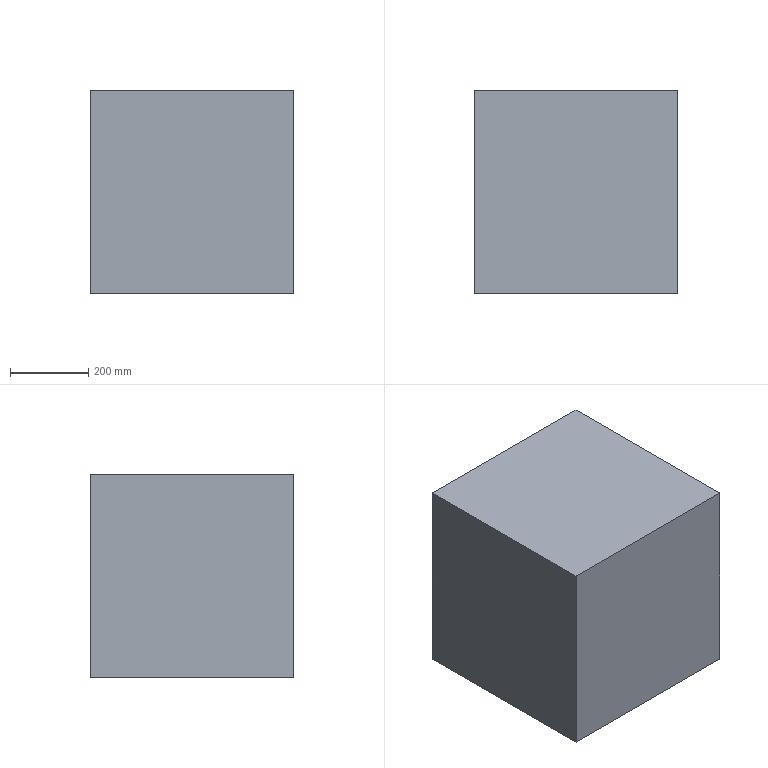Part | SolidWorks | features ICE 2, BaseBody 1 | 1 solid | 44 faces | box 520 x 520 x 520 mm | volume 15406938 mm3 | cylinder 32 | plane 12 | commonest cylinder face diameters 40 x32
STEP:
#1=CARTESIAN_POINT('',(400.507,102.938,240.));
#2=VERTEX_POINT('',#1);
#3=CARTESIAN_POINT('',(400.507,102.938,200.));
#4=VERTEX_POINT('',#3);
#5=CARTESIAN_POINT('',(400.507,102.938,220.));
#6=DIRECTION('',(1.,0.,0.));
#7=DIRECTION('',(0.,0.,-1.));
#8=AXIS2_PLACEMENT_3D('',#5,#6,#7);
#9=CIRCLE('',#8,20.);
#10=EDGE_CURVE('',#2,#4,#9,.T.);
#11=ORIENTED_EDGE('',*,*,#10,.F.);
#12=CARTESIAN_POINT('',(410.507,102.938,240.));
#13=VERTEX_POINT('',#12);
#14=CARTESIAN_POINT('',(400.507,102.938,240.));
#15=DIRECTION('',(1.,0.,0.));
#16=VECTOR('',#15,1000.);
#17=LINE('',#14,#16);
#18=EDGE_CURVE('',#2,#13,#17,.T.);
#19=ORIENTED_EDGE('',*,*,#18,.T.);
#20=CARTESIAN_POINT('',(410.507,102.938,200.));
#21=VERTEX_POINT('',#20);
#22=CARTESIAN_POINT('',(410.507,102.938,220.));
#23=DIRECTION('',(1.,0.,0.));
#24=DIRECTION('',(0.,0.,-1.));
#25=AXIS2_PLACEMENT_3D('',#22,#23,#24);
#26=CIRCLE('',#25,20.);
#27=EDGE_CURVE('',#13,#21,#26,.T.);
#28=ORIENTED_EDGE('',*,*,#27,.T.);
#29=CARTESIAN_POINT('',(400.507,102.938,200.));
#30=DIRECTION('',(1.,0.,0.));
#31=VECTOR('',#30,1000.);
#32=LINE('',#29,#31);
#33=EDGE_CURVE('',#4,#21,#32,.T.);
#34=ORIENTED_EDGE('',*,*,#33,.F.);
#35=EDGE_LOOP('',(#11,#19,#28,#34));
#36=FACE_OUTER_BOUND('',#35,.T.);
#37=CARTESIAN_POINT('',(400.507,102.938,220.));
#38=DIRECTION('',(1.,0.,0.));
#39=DIRECTION('',(0.,0.,-1.));
#40=AXIS2_PLACEMENT_3D('',#37,#38,#39);
#41=CYLINDRICAL_SURFACE('',#40,20.);
#42=ADVANCED_FACE('',(#36),#41,.F.);
#43=CARTESIAN_POINT('',(400.507,102.938,340.));
#44=VERTEX_POINT('',#43);
#45=CARTESIAN_POINT('',(400.507,102.938,300.));
#46=VERTEX_POINT('',#45);
#47=CARTESIAN_POINT('',(400.507,102.938,320.));
#48=DIRECTION('',(1.,0.,0.));
#49=DIRECTION('',(0.,0.,-1.));
#50=AXIS2_PLACEMENT_3D('',#47,#48,#49);
#51=CIRCLE('',#50,20.);
#52=EDGE_CURVE('',#44,#46,#51,.T.);
#53=ORIENTED_EDGE('',*,*,#52,.F.);
#54=CARTESIAN_POINT('',(410.507,102.938,340.));
#55=VERTEX_POINT('',#54);
#56=CARTESIAN_POINT('',(400.507,102.938,340.));
#57=DIRECTION('',(1.,0.,0.));
#58=VECTOR('',#57,1000.);
#59=LINE('',#56,#58);
#60=EDGE_CURVE('',#44,#55,#59,.T.);
#61=ORIENTED_EDGE('',*,*,#60,.T.);
#62=CARTESIAN_POINT('',(410.507,102.938,300.));
#63=VERTEX_POINT('',#62);
#64=CARTESIAN_POINT('',(410.507,102.938,320.));
#65=DIRECTION('',(1.,0.,0.));
#66=DIRECTION('',(0.,0.,-1.));
#67=AXIS2_PLACEMENT_3D('',#64,#65,#66);
#68=CIRCLE('',#67,20.);
#69=EDGE_CURVE('',#55,#63,#68,.T.);
#70=ORIENTED_EDGE('',*,*,#69,.T.);
#71=CARTESIAN_POINT('',(400.507,102.938,300.));
#72=DIRECTION('',(1.,0.,0.));
#73=VECTOR('',#72,1000.);
#74=LINE('',#71,#73);
#75=EDGE_CURVE('',#46,#63,#74,.T.);
#76=ORIENTED_EDGE('',*,*,#75,.F.);
#77=EDGE_LOOP('',(#53,#61,#70,#76));
#78=FACE_OUTER_BOUND('',#77,.T.);
#79=CARTESIAN_POINT('',(400.507,102.938,320.));
#80=DIRECTION('',(1.,0.,0.));
#81=DIRECTION('',(0.,0.,-1.));
#82=AXIS2_PLACEMENT_3D('',#79,#80,#81);
#83=CYLINDRICAL_SURFACE('',#82,20.);
#84=ADVANCED_FACE('',(#78),#83,.F.);
#85=CARTESIAN_POINT('',(400.507,-97.062,440.));
#86=VERTEX_POINT('',#85);
#87=CARTESIAN_POINT('',(400.507,-97.062,400.));
#88=VERTEX_POINT('',#87);
#89=CARTESIAN_POINT('',(400.507,-97.062,420.));
#90=DIRECTION('',(1.,0.,0.));
#91=DIRECTION('',(0.,0.,-1.));
#92=AXIS2_PLACEMENT_3D('',#89,#90,#91);
#93=CIRCLE('',#92,20.);
#94=EDGE_CURVE('',#86,#88,#93,.T.);
#95=ORIENTED_EDGE('',*,*,#94,.F.);
#96=CARTESIAN_POINT('',(410.507,-97.062,440.));
#97=VERTEX_POINT('',#96);
#98=CARTESIAN_POINT('',(400.507,-97.062,440.));
#99=DIRECTION('',(1.,0.,0.));
#100=VECTOR('',#99,1000.);
#101=LINE('',#98,#100);
#102=EDGE_CURVE('',#86,#97,#101,.T.);
#103=ORIENTED_EDGE('',*,*,#102,.T.);
#104=CARTESIAN_POINT('',(410.507,-97.062,400.));
#105=VERTEX_POINT('',#104);
#106=CARTESIAN_POINT('',(410.507,-97.062,420.));
#107=DIRECTION('',(1.,0.,0.));
#108=DIRECTION('',(0.,0.,-1.));
#109=AXIS2_PLACEMENT_3D('',#106,#107,#108);
#110=CIRCLE('',#109,20.);
#111=EDGE_CURVE('',#97,#105,#110,.T.);
#112=ORIENTED_EDGE('',*,*,#111,.T.);
#113=CARTESIAN_POINT('',(400.507,-97.062,400.));
#114=DIRECTION('',(1.,0.,0.));
#115=VECTOR('',#114,1000.);
#116=LINE('',#113,#115);
#117=EDGE_CURVE('',#88,#105,#116,.T.);
#118=ORIENTED_EDGE('',*,*,#117,.F.);
#119=EDGE_LOOP('',(#95,#103,#112,#118));
#120=FACE_OUTER_BOUND('',#119,.T.);
#121=CARTESIAN_POINT('',(400.507,-97.062,420.));
#122=DIRECTION('',(1.,0.,0.));
#123=DIRECTION('',(0.,0.,-1.));
#124=AXIS2_PLACEMENT_3D('',#121,#122,#123);
#125=CYLINDRICAL_SURFACE('',#124,20.);
#126=ADVANCED_FACE('',(#120),#125,.F.);
#127=CARTESIAN_POINT('',(400.507,2.938,440.));
#128=VERTEX_POINT('',#127);
#129=CARTESIAN_POINT('',(400.507,2.938,400.));
#130=VERTEX_POINT('',#129);
#131=CARTESIAN_POINT('',(400.507,2.938,420.));
#132=DIRECTION('',(1.,0.,0.));
#133=DIRECTION('',(0.,0.,-1.));
#134=AXIS2_PLACEMENT_3D('',#131,#132,#133);
#135=CIRCLE('',#134,20.);
#136=EDGE_CURVE('',#128,#130,#135,.T.);
#137=ORIENTED_EDGE('',*,*,#136,.F.);
#138=CARTESIAN_POINT('',(410.507,2.938,440.));
#139=VERTEX_POINT('',#138);
#140=CARTESIAN_POINT('',(400.507,2.938,440.));
#141=DIRECTION('',(1.,0.,0.));
#142=VECTOR('',#141,1000.);
#143=LINE('',#140,#142);
#144=EDGE_CURVE('',#128,#139,#143,.T.);
#145=ORIENTED_EDGE('',*,*,#144,.T.);
#146=CARTESIAN_POINT('',(410.507,2.938,400.));
#147=VERTEX_POINT('',#146);
#148=CARTESIAN_POINT('',(410.507,2.938,420.));
#149=DIRECTION('',(1.,0.,0.));
#150=DIRECTION('',(0.,0.,-1.));
#151=AXIS2_PLACEMENT_3D('',#148,#149,#150);
#152=CIRCLE('',#151,20.);
#153=EDGE_CURVE('',#139,#147,#152,.T.);
#154=ORIENTED_EDGE('',*,*,#153,.T.);
#155=CARTESIAN_POINT('',(400.507,2.938,400.));
#156=DIRECTION('',(1.,0.,0.));
#157=VECTOR('',#156,1000.);
#158=LINE('',#155,#157);
#159=EDGE_CURVE('',#130,#147,#158,.T.);
#160=ORIENTED_EDGE('',*,*,#159,.F.);
#161=EDGE_LOOP('',(#137,#145,#154,#160));
#162=FACE_OUTER_BOUND('',#161,.T.);
#163=CARTESIAN_POINT('',(400.507,2.938,420.));
#164=DIRECTION('',(1.,0.,0.));
#165=DIRECTION('',(0.,0.,-1.));
#166=AXIS2_PLACEMENT_3D('',#163,#164,#165);
#167=CYLINDRICAL_SURFACE('',#166,20.);
#168=ADVANCED_FACE('',(#162),#167,.F.);
#169=CARTESIAN_POINT('',(400.507,202.938,340.));
#170=VERTEX_POINT('',#169);
#171=CARTESIAN_POINT('',(400.507,202.938,300.));
#172=VERTEX_POINT('',#171);
#173=CARTESIAN_POINT('',(400.507,202.938,320.));
#174=DIRECTION('',(1.,0.,0.));
#175=DIRECTION('',(0.,0.,-1.));
#176=AXIS2_PLACEMENT_3D('',#173,#174,#175);
#177=CIRCLE('',#176,20.);
#178=EDGE_CURVE('',#170,#172,#177,.T.);
#179=ORIENTED_EDGE('',*,*,#178,.F.);
#180=CARTESIAN_POINT('',(410.507,202.938,340.));
#181=VERTEX_POINT('',#180);
#182=CARTESIAN_POINT('',(400.507,202.938,340.));
#183=DIRECTION('',(1.,0.,0.));
#184=VECTOR('',#183,1000.);
#185=LINE('',#182,#184);
#186=EDGE_CURVE('',#170,#181,#185,.T.);
#187=ORIENTED_EDGE('',*,*,#186,.T.);
#188=CARTESIAN_POINT('',(410.507,202.938,300.));
#189=VERTEX_POINT('',#188);
#190=CARTESIAN_POINT('',(410.507,202.938,320.));
#191=DIRECTION('',(1.,0.,0.));
#192=DIRECTION('',(0.,0.,-1.));
#193=AXIS2_PLACEMENT_3D('',#190,#191,#192);
#194=CIRCLE('',#193,20.);
#195=EDGE_CURVE('',#181,#189,#194,.T.);
#196=ORIENTED_EDGE('',*,*,#195,.T.);
#197=CARTESIAN_POINT('',(400.507,202.938,300.));
#198=DIRECTION('',(1.,0.,0.));
#199=VECTOR('',#198,1000.);
#200=LINE('',#197,#199);
#201=EDGE_CURVE('',#172,#189,#200,.T.);
#202=ORIENTED_EDGE('',*,*,#201,.F.);
#203=EDGE_LOOP('',(#179,#187,#196,#202));
#204=FACE_OUTER_BOUND('',#203,.T.);
#205=CARTESIAN_POINT('',(400.507,202.938,320.));
#206=DIRECTION('',(1.,0.,0.));
#207=DIRECTION('',(0.,0.,-1.));
#208=AXIS2_PLACEMENT_3D('',#205,#206,#207);
#209=CYLINDRICAL_SURFACE('',#208,20.);
#210=ADVANCED_FACE('',(#204),#209,.F.);
#211=CARTESIAN_POINT('',(400.507,202.938,240.));
#212=VERTEX_POINT('',#211);
#213=CARTESIAN_POINT('',(400.507,202.938,200.));
#214=VERTEX_POINT('',#213);
#215=CARTESIAN_POINT('',(400.507,202.938,220.));
#216=DIRECTION('',(1.,0.,0.));
#217=DIRECTION('',(0.,0.,-1.));
#218=AXIS2_PLACEMENT_3D('',#215,#216,#217);
#219=CIRCLE('',#218,20.);
#220=EDGE_CURVE('',#212,#214,#219,.T.);
#221=ORIENTED_EDGE('',*,*,#220,.F.);
#222=CARTESIAN_POINT('',(410.507,202.938,240.));
#223=VERTEX_POINT('',#222);
#224=CARTESIAN_POINT('',(400.507,202.938,240.));
#225=DIRECTION('',(1.,0.,0.));
#226=VECTOR('',#225,1000.);
#227=LINE('',#224,#226);
#228=EDGE_CURVE('',#212,#223,#227,.T.);
#229=ORIENTED_EDGE('',*,*,#228,.T.);
#230=CARTESIAN_POINT('',(410.507,202.938,200.));
#231=VERTEX_POINT('',#230);
#232=CARTESIAN_POINT('',(410.507,202.938,220.));
#233=DIRECTION('',(1.,0.,0.));
#234=DIRECTION('',(0.,0.,-1.));
#235=AXIS2_PLACEMENT_3D('',#232,#233,#234);
#236=CIRCLE('',#235,20.);
#237=EDGE_CURVE('',#223,#231,#236,.T.);
#238=ORIENTED_EDGE('',*,*,#237,.T.);
#239=CARTESIAN_POINT('',(400.507,202.938,200.));
#240=DIRECTION('',(1.,0.,0.));
#241=VECTOR('',#240,1000.);
#242=LINE('',#239,#241);
#243=EDGE_CURVE('',#214,#231,#242,.T.);
#244=ORIENTED_EDGE('',*,*,#243,.F.);
#245=EDGE_LOOP('',(#221,#229,#238,#244));
#246=FACE_OUTER_BOUND('',#245,.T.);
#247=CARTESIAN_POINT('',(400.507,202.938,220.));
#248=DIRECTION('',(1.,0.,0.));
#249=DIRECTION('',(0.,0.,-1.));
#250=AXIS2_PLACEMENT_3D('',#247,#248,#249);
#251=CYLINDRICAL_SURFACE('',#250,20.);
#252=ADVANCED_FACE('',(#246),#251,.F.);
#253=CARTESIAN_POINT('',(400.507,202.938,140.));
#254=VERTEX_POINT('',#253);
#255=CARTESIAN_POINT('',(400.507,202.938,100.));
#256=VERTEX_POINT('',#255);
#257=CARTESIAN_POINT('',(400.507,202.938,120.));
#258=DIRECTION('',(1.,0.,0.));
#259=DIRECTION('',(0.,0.,-1.));
#260=AXIS2_PLACEMENT_3D('',#257,#258,#259);
#261=CIRCLE('',#260,20.);
#262=EDGE_CURVE('',#254,#256,#261,.T.);
#263=ORIENTED_EDGE('',*,*,#262,.F.);
#264=CARTESIAN_POINT('',(410.507,202.938,140.));
#265=VERTEX_POINT('',#264);
#266=CARTESIAN_POINT('',(400.507,202.938,140.));
#267=DIRECTION('',(1.,0.,0.));
#268=VECTOR('',#267,1000.);
#269=LINE('',#266,#268);
#270=EDGE_CURVE('',#254,#265,#269,.T.);
#271=ORIENTED_EDGE('',*,*,#270,.T.);
#272=CARTESIAN_POINT('',(410.507,202.938,100.));
#273=VERTEX_POINT('',#272);
#274=CARTESIAN_POINT('',(410.507,202.938,120.));
#275=DIRECTION('',(1.,0.,0.));
#276=DIRECTION('',(0.,0.,-1.));
#277=AXIS2_PLACEMENT_3D('',#274,#275,#276);
#278=CIRCLE('',#277,20.);
#279=EDGE_CURVE('',#265,#273,#278,.T.);
#280=ORIENTED_EDGE('',*,*,#279,.T.);
#281=CARTESIAN_POINT('',(400.507,202.938,100.));
#282=DIRECTION('',(1.,0.,0.));
#283=VECTOR('',#282,1000.);
#284=LINE('',#281,#283);
#285=EDGE_CURVE('',#256,#273,#284,.T.);
#286=ORIENTED_EDGE('',*,*,#285,.F.);
#287=EDGE_LOOP('',(#263,#271,#280,#286));
#288=FACE_OUTER_BOUND('',#287,.T.);
#289=CARTESIAN_POINT('',(400.507,202.938,120.));
#290=DIRECTION('',(1.,0.,0.));
#291=DIRECTION('',(0.,0.,-1.));
#292=AXIS2_PLACEMENT_3D('',#289,#290,#291);
#293=CYLINDRICAL_SURFACE('',#292,20.);
#294=ADVANCED_FACE('',(#288),#293,.F.);
#295=CARTESIAN_POINT('',(400.507,102.938,440.));
#296=VERTEX_POINT('',#295);
#297=CARTESIAN_POINT('',(400.507,102.938,400.));
#298=VERTEX_POINT('',#297);
#299=CARTESIAN_POINT('',(400.507,102.938,420.));
#300=DIRECTION('',(1.,0.,0.));
#301=DIRECTION('',(0.,0.,-1.));
#302=AXIS2_PLACEMENT_3D('',#299,#300,#301);
#303=CIRCLE('',#302,20.);
#304=EDGE_CURVE('',#296,#298,#303,.T.);
#305=ORIENTED_EDGE('',*,*,#304,.F.);
#306=CARTESIAN_POINT('',(410.507,102.938,440.));
#307=VERTEX_POINT('',#306);
#308=CARTESIAN_POINT('',(400.507,102.938,440.));
#309=DIRECTION('',(1.,0.,0.));
#310=VECTOR('',#309,1000.);
#311=LINE('',#308,#310);
#312=EDGE_CURVE('',#296,#307,#311,.T.);
#313=ORIENTED_EDGE('',*,*,#312,.T.);
#314=CARTESIAN_POINT('',(410.507,102.938,400.));
#315=VERTEX_POINT('',#314);
#316=CARTESIAN_POINT('',(410.507,102.938,420.));
#317=DIRECTION('',(1.,0.,0.));
#318=DIRECTION('',(0.,0.,-1.));
#319=AXIS2_PLACEMENT_3D('',#316,#317,#318);
#320=CIRCLE('',#319,20.);
#321=EDGE_CURVE('',#307,#315,#320,.T.);
#322=ORIENTED_EDGE('',*,*,#321,.T.);
#323=CARTESIAN_POINT('',(400.507,102.938,400.));
#324=DIRECTION('',(1.,0.,0.));
#325=VECTOR('',#324,1000.);
#326=LINE('',#323,#325);
#327=EDGE_CURVE('',#298,#315,#326,.T.);
#328=ORIENTED_EDGE('',*,*,#327,.F.);
#329=EDGE_LOOP('',(#305,#313,#322,#328));
#330=FACE_OUTER_BOUND('',#329,.T.);
#331=CARTESIAN_POINT('',(400.507,102.938,420.));
#332=DIRECTION('',(1.,0.,0.));
#333=DIRECTION('',(0.,0.,-1.));
#334=AXIS2_PLACEMENT_3D('',#331,#332,#333);
#335=CYLINDRICAL_SURFACE('',#334,20.);
#336=ADVANCED_FACE('',(#330),#335,.F.);
#337=CARTESIAN_POINT('',(400.507,2.938,140.));
#338=VERTEX_POINT('',#337);
#339=CARTESIAN_POINT('',(400.507,2.938,100.));
#340=VERTEX_POINT('',#339);
#341=CARTESIAN_POINT('',(400.507,2.938,120.));
#342=DIRECTION('',(1.,0.,0.));
#343=DIRECTION('',(0.,0.,-1.));
#344=AXIS2_PLACEMENT_3D('',#341,#342,#343);
#345=CIRCLE('',#344,20.);
#346=EDGE_CURVE('',#338,#340,#345,.T.);
#347=ORIENTED_EDGE('',*,*,#346,.F.);
#348=CARTESIAN_POINT('',(410.507,2.938,140.));
#349=VERTEX_POINT('',#348);
#350=CARTESIAN_POINT('',(400.507,2.938,140.));
#351=DIRECTION('',(1.,0.,0.));
#352=VECTOR('',#351,1000.);
#353=LINE('',#350,#352);
#354=EDGE_CURVE('',#338,#349,#353,.T.);
#355=ORIENTED_EDGE('',*,*,#354,.T.);
#356=CARTESIAN_POINT('',(410.507,2.938,100.));
#357=VERTEX_POINT('',#356);
#358=CARTESIAN_POINT('',(410.507,2.938,120.));
#359=DIRECTION('',(1.,0.,0.));
#360=DIRECTION('',(0.,0.,-1.));
#361=AXIS2_PLACEMENT_3D('',#358,#359,#360);
#362=CIRCLE('',#361,20.);
#363=EDGE_CURVE('',#349,#357,#362,.T.);
#364=ORIENTED_EDGE('',*,*,#363,.T.);
#365=CARTESIAN_POINT('',(400.507,2.938,100.));
#366=DIRECTION('',(1.,0.,0.));
#367=VECTOR('',#366,1000.);
#368=LINE('',#365,#367);
#369=EDGE_CURVE('',#340,#357,#368,.T.);
#370=ORIENTED_EDGE('',*,*,#369,.F.);
#371=EDGE_LOOP('',(#347,#355,#364,#370));
#372=FACE_OUTER_BOUND('',#371,.T.);
#373=CARTESIAN_POINT('',(400.507,2.938,120.));
#374=DIRECTION('',(1.,0.,0.));
#375=DIRECTION('',(0.,0.,-1.));
#376=AXIS2_PLACEMENT_3D('',#373,#374,#375);
#377=CYLINDRICAL_SURFACE('',#376,20.);
#378=ADVANCED_FACE('',(#372),#377,.F.);
#379=CARTESIAN_POINT('',(400.507,2.938,240.));
#380=VERTEX_POINT('',#379);
#381=CARTESIAN_POINT('',(400.507,2.938,200.));
#382=VERTEX_POINT('',#381);
#383=CARTESIAN_POINT('',(400.507,2.938,220.));
#384=DIRECTION('',(1.,0.,0.));
#385=DIRECTION('',(0.,0.,-1.));
#386=AXIS2_PLACEMENT_3D('',#383,#384,#385);
#387=CIRCLE('',#386,20.);
#388=EDGE_CURVE('',#380,#382,#387,.T.);
#389=ORIENTED_EDGE('',*,*,#388,.F.);
#390=CARTESIAN_POINT('',(410.507,2.938,240.));
#391=VERTEX_POINT('',#390);
#392=CARTESIAN_POINT('',(400.507,2.938,240.));
#393=DIRECTION('',(1.,0.,0.));
#394=VECTOR('',#393,1000.);
#395=LINE('',#392,#394);
#396=EDGE_CURVE('',#380,#391,#395,.T.);
#397=ORIENTED_EDGE('',*,*,#396,.T.);
#398=CARTESIAN_POINT('',(410.507,2.938,200.));
#399=VERTEX_POINT('',#398);
#400=CARTESIAN_POINT('',(410.507,2.938,220.));
#401=DIRECTION('',(1.,0.,0.));
#402=DIRECTION('',(0.,0.,-1.));
#403=AXIS2_PLACEMENT_3D('',#400,#401,#402);
#404=CIRCLE('',#403,20.);
#405=EDGE_CURVE('',#391,#399,#404,.T.);
#406=ORIENTED_EDGE('',*,*,#405,.T.);
#407=CARTESIAN_POINT('',(400.507,2.938,200.));
#408=DIRECTION('',(1.,0.,0.));
#409=VECTOR('',#408,1000.);
#410=LINE('',#407,#409);
#411=EDGE_CURVE('',#382,#399,#410,.T.);
#412=ORIENTED_EDGE('',*,*,#411,.F.);
#413=EDGE_LOOP('',(#389,#397,#406,#412));
#414=FACE_OUTER_BOUND('',#413,.T.);
#415=CARTESIAN_POINT('',(400.507,2.938,220.));
#416=DIRECTION('',(1.,0.,0.));
#417=DIRECTION('',(0.,0.,-1.));
#418=AXIS2_PLACEMENT_3D('',#415,#416,#417);
#419=CYLINDRICAL_SURFACE('',#418,20.);
#420=ADVANCED_FACE('',(#414),#419,.F.);
#421=CARTESIAN_POINT('',(400.507,2.938,340.));
#422=VERTEX_POINT('',#421);
#423=CARTESIAN_POINT('',(400.507,2.938,300.));
#424=VERTEX_POINT('',#423);
#425=CARTESIAN_POINT('',(400.507,2.938,320.));
#426=DIRECTION('',(1.,0.,0.));
#427=DIRECTION('',(0.,0.,-1.));
#428=AXIS2_PLACEMENT_3D('',#425,#426,#427);
#429=CIRCLE('',#428,20.);
#430=EDGE_CURVE('',#422,#424,#429,.T.);
#431=ORIENTED_EDGE('',*,*,#430,.F.);
#432=CARTESIAN_POINT('',(410.507,2.938,340.));
#433=VERTEX_POINT('',#432);
#434=CARTESIAN_POINT('',(400.507,2.938,340.));
#435=DIRECTION('',(1.,0.,0.));
#436=VECTOR('',#435,1000.);
#437=LINE('',#434,#436);
#438=EDGE_CURVE('',#422,#433,#437,.T.);
#439=ORIENTED_EDGE('',*,*,#438,.T.);
#440=CARTESIAN_POINT('',(410.507,2.938,300.));
#441=VERTEX_POINT('',#440);
#442=CARTESIAN_POINT('',(410.507,2.938,320.));
#443=DIRECTION('',(1.,0.,0.));
#444=DIRECTION('',(0.,0.,-1.));
#445=AXIS2_PLACEMENT_3D('',#442,#443,#444);
#446=CIRCLE('',#445,20.);
#447=EDGE_CURVE('',#433,#441,#446,.T.);
#448=ORIENTED_EDGE('',*,*,#447,.T.);
#449=CARTESIAN_POINT('',(400.507,2.938,300.));
#450=DIRECTION('',(1.,0.,0.));
#451=VECTOR('',#450,1000.);
#452=LINE('',#449,#451);
#453=EDGE_CURVE('',#424,#441,#452,.T.);
#454=ORIENTED_EDGE('',*,*,#453,.F.);
#455=EDGE_LOOP('',(#431,#439,#448,#454));
#456=FACE_OUTER_BOUND('',#455,.T.);
#457=CARTESIAN_POINT('',(400.507,2.938,320.));
#458=DIRECTION('',(1.,0.,0.));
#459=DIRECTION('',(0.,0.,-1.));
#460=AXIS2_PLACEMENT_3D('',#457,#458,#459);
#461=CYLINDRICAL_SURFACE('',#460,20.);
#462=ADVANCED_FACE('',(#456),#461,.F.);
#463=CARTESIAN_POINT('',(400.507,102.938,140.));
#464=VERTEX_POINT('',#463);
#465=CARTESIAN_POINT('',(400.507,102.938,100.));
#466=VERTEX_POINT('',#465);
#467=CARTESIAN_POINT('',(400.507,102.938,120.));
#468=DIRECTION('',(1.,0.,0.));
#469=DIRECTION('',(0.,0.,-1.));
#470=AXIS2_PLACEMENT_3D('',#467,#468,#469);
#471=CIRCLE('',#470,20.);
#472=EDGE_CURVE('',#464,#466,#471,.T.);
#473=ORIENTED_EDGE('',*,*,#472,.F.);
#474=CARTESIAN_POINT('',(410.507,102.938,140.));
#475=VERTEX_POINT('',#474);
#476=CARTESIAN_POINT('',(400.507,102.938,140.));
#477=DIRECTION('',(1.,0.,0.));
#478=VECTOR('',#477,1000.);
#479=LINE('',#476,#478);
#480=EDGE_CURVE('',#464,#475,#479,.T.);
#481=ORIENTED_EDGE('',*,*,#480,.T.);
#482=CARTESIAN_POINT('',(410.507,102.938,100.));
#483=VERTEX_POINT('',#482);
#484=CARTESIAN_POINT('',(410.507,102.938,120.));
#485=DIRECTION('',(1.,0.,0.));
#486=DIRECTION('',(0.,0.,-1.));
#487=AXIS2_PLACEMENT_3D('',#484,#485,#486);
#488=CIRCLE('',#487,20.);
#489=EDGE_CURVE('',#475,#483,#488,.T.);
#490=ORIENTED_EDGE('',*,*,#489,.T.);
#491=CARTESIAN_POINT('',(400.507,102.938,100.));
#492=DIRECTION('',(1.,0.,0.));
#493=VECTOR('',#492,1000.);
#494=LINE('',#491,#493);
#495=EDGE_CURVE('',#466,#483,#494,.T.);
#496=ORIENTED_EDGE('',*,*,#495,.F.);
#497=EDGE_LOOP('',(#473,#481,#490,#496));
#498=FACE_OUTER_BOUND('',#497,.T.);
#499=CARTESIAN_POINT('',(400.507,102.938,120.));
#500=DIRECTION('',(1.,0.,0.));
#501=DIRECTION('',(0.,0.,-1.));
#502=AXIS2_PLACEMENT_3D('',#499,#500,#501);
#503=CYLINDRICAL_SURFACE('',#502,20.);
#504=ADVANCED_FACE('',(#498),#503,.F.);
#505=CARTESIAN_POINT('',(400.507,-97.062,340.));
#506=VERTEX_POINT('',#505);
#507=CARTESIAN_POINT('',(400.507,-97.062,300.));
#508=VERTEX_POINT('',#507);
#509=CARTESIAN_POINT('',(400.507,-97.062,320.));
#510=DIRECTION('',(1.,0.,0.));
#511=DIRECTION('',(0.,0.,-1.));
#512=AXIS2_PLACEMENT_3D('',#509,#510,#511);
#513=CIRCLE('',#512,20.);
#514=EDGE_CURVE('',#506,#508,#513,.T.);
#515=ORIENTED_EDGE('',*,*,#514,.F.);
#516=CARTESIAN_POINT('',(410.507,-97.062,340.));
#517=VERTEX_POINT('',#516);
#518=CARTESIAN_POINT('',(400.507,-97.062,340.));
#519=DIRECTION('',(1.,0.,0.));
#520=VECTOR('',#519,1000.);
#521=LINE('',#518,#520);
#522=EDGE_CURVE('',#506,#517,#521,.T.);
#523=ORIENTED_EDGE('',*,*,#522,.T.);
#524=CARTESIAN_POINT('',(410.507,-97.062,300.));
#525=VERTEX_POINT('',#524);
#526=CARTESIAN_POINT('',(410.507,-97.062,320.));
#527=DIRECTION('',(1.,0.,0.));
#528=DIRECTION('',(0.,0.,-1.));
#529=AXIS2_PLACEMENT_3D('',#526,#527,#528);
#530=CIRCLE('',#529,20.);
#531=EDGE_CURVE('',#517,#525,#530,.T.);
#532=ORIENTED_EDGE('',*,*,#531,.T.);
#533=CARTESIAN_POINT('',(400.507,-97.062,300.));
#534=DIRECTION('',(1.,0.,0.));
#535=VECTOR('',#534,1000.);
#536=LINE('',#533,#535);
#537=EDGE_CURVE('',#508,#525,#536,.T.);
#538=ORIENTED_EDGE('',*,*,#537,.F.);
#539=EDGE_LOOP('',(#515,#523,#532,#538));
#540=FACE_OUTER_BOUND('',#539,.T.);
#541=CARTESIAN_POINT('',(400.507,-97.062,320.));
#542=DIRECTION('',(1.,0.,0.));
#543=DIRECTION('',(0.,0.,-1.));
#544=AXIS2_PLACEMENT_3D('',#541,#542,#543);
#545=CYLINDRICAL_SURFACE('',#544,20.);
#546=ADVANCED_FACE('',(#540),#545,.F.);
#547=CARTESIAN_POINT('',(400.507,-97.062,240.));
#548=VERTEX_POINT('',#547);
#549=CARTESIAN_POINT('',(400.507,-97.062,200.));
#550=VERTEX_POINT('',#549);
#551=CARTESIAN_POINT('',(400.507,-97.062,220.));
#552=DIRECTION('',(1.,0.,0.));
#553=DIRECTION('',(0.,0.,-1.));
#554=AXIS2_PLACEMENT_3D('',#551,#552,#553);
#555=CIRCLE('',#554,20.);
#556=EDGE_CURVE('',#548,#550,#555,.T.);
#557=ORIENTED_EDGE('',*,*,#556,.F.);
#558=CARTESIAN_POINT('',(410.507,-97.062,240.));
#559=VERTEX_POINT('',#558);
#560=CARTESIAN_POINT('',(400.507,-97.062,240.));
#561=DIRECTION('',(1.,0.,0.));
#562=VECTOR('',#561,1000.);
#563=LINE('',#560,#562);
#564=EDGE_CURVE('',#548,#559,#563,.T.);
#565=ORIENTED_EDGE('',*,*,#564,.T.);
#566=CARTESIAN_POINT('',(410.507,-97.062,200.));
#567=VERTEX_POINT('',#566);
#568=CARTESIAN_POINT('',(410.507,-97.062,220.));
#569=DIRECTION('',(1.,0.,0.));
#570=DIRECTION('',(0.,0.,-1.));
#571=AXIS2_PLACEMENT_3D('',#568,#569,#570);
#572=CIRCLE('',#571,20.);
#573=EDGE_CURVE('',#559,#567,#572,.T.);
#574=ORIENTED_EDGE('',*,*,#573,.T.);
#575=CARTESIAN_POINT('',(400.507,-97.062,200.));
#576=DIRECTION('',(1.,0.,0.));
#577=VECTOR('',#576,1000.);
#578=LINE('',#575,#577);
#579=EDGE_CURVE('',#550,#567,#578,.T.);
#580=ORIENTED_EDGE('',*,*,#579,.F.);
#581=EDGE_LOOP('',(#557,#565,#574,#580));
#582=FACE_OUTER_BOUND('',#581,.T.);
#583=CARTESIAN_POINT('',(400.507,-97.062,220.));
#584=DIRECTION('',(1.,0.,0.));
#585=DIRECTION('',(0.,0.,-1.));
#586=AXIS2_PLACEMENT_3D('',#583,#584,#585);
#587=CYLINDRICAL_SURFACE('',#586,20.);
#588=ADVANCED_FACE('',(#582),#587,.F.);
#589=CARTESIAN_POINT('',(400.507,-97.062,140.));
#590=VERTEX_POINT('',#589);
#591=CARTESIAN_POINT('',(400.507,-97.062,100.));
#592=VERTEX_POINT('',#591);
#593=CARTESIAN_POINT('',(400.507,-97.062,120.));
#594=DIRECTION('',(1.,0.,0.));
#595=DIRECTION('',(0.,0.,-1.));
#596=AXIS2_PLACEMENT_3D('',#593,#594,#595);
#597=CIRCLE('',#596,20.);
#598=EDGE_CURVE('',#590,#592,#597,.T.);
#599=ORIENTED_EDGE('',*,*,#598,.F.);
#600=CARTESIAN_POINT('',(410.507,-97.062,140.));
#601=VERTEX_POINT('',#600);
#602=CARTESIAN_POINT('',(400.507,-97.062,140.));
#603=DIRECTION('',(1.,0.,0.));
#604=VECTOR('',#603,1000.);
#605=LINE('',#602,#604);
#606=EDGE_CURVE('',#590,#601,#605,.T.);
#607=ORIENTED_EDGE('',*,*,#606,.T.);
#608=CARTESIAN_POINT('',(410.507,-97.062,100.));
#609=VERTEX_POINT('',#608);
#610=CARTESIAN_POINT('',(410.507,-97.062,120.));
#611=DIRECTION('',(1.,0.,0.));
#612=DIRECTION('',(0.,0.,-1.));
#613=AXIS2_PLACEMENT_3D('',#610,#611,#612);
#614=CIRCLE('',#613,20.);
#615=EDGE_CURVE('',#601,#609,#614,.T.);
#616=ORIENTED_EDGE('',*,*,#615,.T.);
#617=CARTESIAN_POINT('',(400.507,-97.062,100.));
#618=DIRECTION('',(1.,0.,0.));
#619=VECTOR('',#618,1000.);
#620=LINE('',#617,#619);
#621=EDGE_CURVE('',#592,#609,#620,.T.);
#622=ORIENTED_EDGE('',*,*,#621,.F.);
#623=EDGE_LOOP('',(#599,#607,#616,#622));
#624=FACE_OUTER_BOUND('',#623,.T.);
#625=CARTESIAN_POINT('',(400.507,-97.062,120.));
#626=DIRECTION('',(1.,0.,0.));
#627=DIRECTION('',(0.,0.,-1.));
#628=AXIS2_PLACEMENT_3D('',#625,#626,#627);
#629=CYLINDRICAL_SURFACE('',#628,20.);
#630=ADVANCED_FACE('',(#624),#629,.F.);
#631=CARTESIAN_POINT('',(400.507,202.938,440.));
#632=VERTEX_POINT('',#631);
#633=CARTESIAN_POINT('',(400.507,202.938,400.));
#634=VERTEX_POINT('',#633);
#635=CARTESIAN_POINT('',(400.507,202.938,420.));
#636=DIRECTION('',(1.,0.,0.));
#637=DIRECTION('',(0.,0.,-1.));
#638=AXIS2_PLACEMENT_3D('',#635,#636,#637);
#639=CIRCLE('',#638,20.);
#640=EDGE_CURVE('',#632,#634,#639,.T.);
#641=ORIENTED_EDGE('',*,*,#640,.F.);
#642=CARTESIAN_POINT('',(410.507,202.938,440.));
#643=VERTEX_POINT('',#642);
#644=CARTESIAN_POINT('',(400.507,202.938,440.));
#645=DIRECTION('',(1.,0.,0.));
#646=VECTOR('',#645,1000.);
#647=LINE('',#644,#646);
#648=EDGE_CURVE('',#632,#643,#647,.T.);
#649=ORIENTED_EDGE('',*,*,#648,.T.);
#650=CARTESIAN_POINT('',(410.507,202.938,400.));
#651=VERTEX_POINT('',#650);
#652=CARTESIAN_POINT('',(410.507,202.938,420.));
#653=DIRECTION('',(1.,0.,0.));
#654=DIRECTION('',(0.,0.,-1.));
#655=AXIS2_PLACEMENT_3D('',#652,#653,#654);
#656=CIRCLE('',#655,20.);
#657=EDGE_CURVE('',#643,#651,#656,.T.);
#658=ORIENTED_EDGE('',*,*,#657,.T.);
#659=CARTESIAN_POINT('',(400.507,202.938,400.));
#660=DIRECTION('',(1.,0.,0.));
#661=VECTOR('',#660,1000.);
#662=LINE('',#659,#661);
#663=EDGE_CURVE('',#634,#651,#662,.T.);
#664=ORIENTED_EDGE('',*,*,#663,.F.);
#665=EDGE_LOOP('',(#641,#649,#658,#664));
#666=FACE_OUTER_BOUND('',#665,.T.);
#667=CARTESIAN_POINT('',(400.507,202.938,420.));
#668=DIRECTION('',(1.,0.,0.));
#669=DIRECTION('',(0.,0.,-1.));
#670=AXIS2_PLACEMENT_3D('',#667,#668,#669);
#671=CYLINDRICAL_SURFACE('',#670,20.);
#672=ADVANCED_FACE('',(#666),#671,.F.);
#673=CARTESIAN_POINT('',(400.507,102.938,220.));
#674=DIRECTION('',(1.,0.,0.));
#675=DIRECTION('',(0.,0.,-1.));
#676=AXIS2_PLACEMENT_3D('',#673,#674,#675);
#677=CIRCLE('',#676,20.);
#678=EDGE_CURVE('',#4,#2,#677,.T.);
#679=ORIENTED_EDGE('',*,*,#678,.T.);
#680=ORIENTED_EDGE('',*,*,#10,.T.);
#681=EDGE_LOOP('',(#679,#680));
#682=FACE_BOUND('',#681,.T.);
#683=CARTESIAN_POINT('',(400.507,102.938,320.));
#684=DIRECTION('',(1.,0.,0.));
#685=DIRECTION('',(0.,0.,-1.));
#686=AXIS2_PLACEMENT_3D('',#683,#684,#685);
#687=CIRCLE('',#686,20.);
#688=EDGE_CURVE('',#46,#44,#687,.T.);
#689=ORIENTED_EDGE('',*,*,#688,.T.);
#690=ORIENTED_EDGE('',*,*,#52,.T.);
#691=EDGE_LOOP('',(#689,#690));
#692=FACE_BOUND('',#691,.T.);
#693=CARTESIAN_POINT('',(400.507,-97.062,420.));
#694=DIRECTION('',(1.,0.,0.));
#695=DIRECTION('',(0.,0.,-1.));
#696=AXIS2_PLACEMENT_3D('',#693,#694,#695);
#697=CIRCLE('',#696,20.);
#698=EDGE_CURVE('',#88,#86,#697,.T.);
#699=ORIENTED_EDGE('',*,*,#698,.T.);
#700=ORIENTED_EDGE('',*,*,#94,.T.);
#701=EDGE_LOOP('',(#699,#700));
#702=FACE_BOUND('',#701,.T.);
#703=CARTESIAN_POINT('',(400.507,2.938,420.));
#704=DIRECTION('',(1.,0.,0.));
#705=DIRECTION('',(0.,0.,-1.));
#706=AXIS2_PLACEMENT_3D('',#703,#704,#705);
#707=CIRCLE('',#706,20.);
#708=EDGE_CURVE('',#130,#128,#707,.T.);
#709=ORIENTED_EDGE('',*,*,#708,.T.);
#710=ORIENTED_EDGE('',*,*,#136,.T.);
#711=EDGE_LOOP('',(#709,#710));
#712=FACE_BOUND('',#711,.T.);
#713=CARTESIAN_POINT('',(400.507,202.938,320.));
#714=DIRECTION('',(1.,0.,0.));
#715=DIRECTION('',(0.,0.,-1.));
#716=AXIS2_PLACEMENT_3D('',#713,#714,#715);
#717=CIRCLE('',#716,20.);
#718=EDGE_CURVE('',#172,#170,#717,.T.);
#719=ORIENTED_EDGE('',*,*,#718,.T.);
#720=ORIENTED_EDGE('',*,*,#178,.T.);
#721=EDGE_LOOP('',(#719,#720));
#722=FACE_BOUND('',#721,.T.);
#723=CARTESIAN_POINT('',(400.507,202.938,220.));
#724=DIRECTION('',(1.,0.,0.));
#725=DIRECTION('',(0.,0.,-1.));
#726=AXIS2_PLACEMENT_3D('',#723,#724,#725);
#727=CIRCLE('',#726,20.);
#728=EDGE_CURVE('',#214,#212,#727,.T.);
#729=ORIENTED_EDGE('',*,*,#728,.T.);
#730=ORIENTED_EDGE('',*,*,#220,.T.);
#731=EDGE_LOOP('',(#729,#730));
#732=FACE_BOUND('',#731,.T.);
#733=CARTESIAN_POINT('',(400.507,202.938,120.));
#734=DIRECTION('',(1.,0.,0.));
#735=DIRECTION('',(0.,0.,-1.));
#736=AXIS2_PLACEMENT_3D('',#733,#734,#735);
#737=CIRCLE('',#736,20.);
#738=EDGE_CURVE('',#256,#254,#737,.T.);
#739=ORIENTED_EDGE('',*,*,#738,.T.);
#740=ORIENTED_EDGE('',*,*,#262,.T.);
#741=EDGE_LOOP('',(#739,#740));
#742=FACE_BOUND('',#741,.T.);
#743=CARTESIAN_POINT('',(400.507,102.938,420.));
#744=DIRECTION('',(1.,0.,0.));
#745=DIRECTION('',(0.,0.,-1.));
#746=AXIS2_PLACEMENT_3D('',#743,#744,#745);
#747=CIRCLE('',#746,20.);
#748=EDGE_CURVE('',#298,#296,#747,.T.);
#749=ORIENTED_EDGE('',*,*,#748,.T.);
#750=ORIENTED_EDGE('',*,*,#304,.T.);
#751=EDGE_LOOP('',(#749,#750));
#752=FACE_BOUND('',#751,.T.);
#753=CARTESIAN_POINT('',(400.507,2.938,120.));
#754=DIRECTION('',(1.,0.,0.));
#755=DIRECTION('',(0.,0.,-1.));
#756=AXIS2_PLACEMENT_3D('',#753,#754,#755);
#757=CIRCLE('',#756,20.);
#758=EDGE_CURVE('',#340,#338,#757,.T.);
#759=ORIENTED_EDGE('',*,*,#758,.T.);
#760=ORIENTED_EDGE('',*,*,#346,.T.);
#761=EDGE_LOOP('',(#759,#760));
#762=FACE_BOUND('',#761,.T.);
#763=CARTESIAN_POINT('',(400.507,2.938,220.));
#764=DIRECTION('',(1.,0.,0.));
#765=DIRECTION('',(0.,0.,-1.));
#766=AXIS2_PLACEMENT_3D('',#763,#764,#765);
#767=CIRCLE('',#766,20.);
#768=EDGE_CURVE('',#382,#380,#767,.T.);
#769=ORIENTED_EDGE('',*,*,#768,.T.);
#770=ORIENTED_EDGE('',*,*,#388,.T.);
#771=EDGE_LOOP('',(#769,#770));
#772=FACE_BOUND('',#771,.T.);
#773=CARTESIAN_POINT('',(400.507,2.938,320.));
#774=DIRECTION('',(1.,0.,0.));
#775=DIRECTION('',(0.,0.,-1.));
#776=AXIS2_PLACEMENT_3D('',#773,#774,#775);
#777=CIRCLE('',#776,20.);
#778=EDGE_CURVE('',#424,#422,#777,.T.);
#779=ORIENTED_EDGE('',*,*,#778,.T.);
#780=ORIENTED_EDGE('',*,*,#430,.T.);
#781=EDGE_LOOP('',(#779,#780));
#782=FACE_BOUND('',#781,.T.);
#783=CARTESIAN_POINT('',(400.507,102.938,120.));
#784=DIRECTION('',(1.,0.,0.));
#785=DIRECTION('',(0.,0.,-1.));
#786=AXIS2_PLACEMENT_3D('',#783,#784,#785);
#787=CIRCLE('',#786,20.);
#788=EDGE_CURVE('',#466,#464,#787,.T.);
#789=ORIENTED_EDGE('',*,*,#788,.T.);
#790=ORIENTED_EDGE('',*,*,#472,.T.);
#791=EDGE_LOOP('',(#789,#790));
#792=FACE_BOUND('',#791,.T.);
#793=CARTESIAN_POINT('',(400.507,-97.062,320.));
#794=DIRECTION('',(1.,0.,0.));
#795=DIRECTION('',(0.,0.,-1.));
#796=AXIS2_PLACEMENT_3D('',#793,#794,#795);
#797=CIRCLE('',#796,20.);
#798=EDGE_CURVE('',#508,#506,#797,.T.);
#799=ORIENTED_EDGE('',*,*,#798,.T.);
#800=ORIENTED_EDGE('',*,*,#514,.T.);
#801=EDGE_LOOP('',(#799,#800));
#802=FACE_BOUND('',#801,.T.);
#803=CARTESIAN_POINT('',(400.507,-97.062,220.));
#804=DIRECTION('',(1.,0.,0.));
#805=DIRECTION('',(0.,0.,-1.));
#806=AXIS2_PLACEMENT_3D('',#803,#804,#805);
#807=CIRCLE('',#806,20.);
#808=EDGE_CURVE('',#550,#548,#807,.T.);
#809=ORIENTED_EDGE('',*,*,#808,.T.);
#810=ORIENTED_EDGE('',*,*,#556,.T.);
#811=EDGE_LOOP('',(#809,#810));
#812=FACE_BOUND('',#811,.T.);
#813=CARTESIAN_POINT('',(400.507,-97.062,120.));
#814=DIRECTION('',(1.,0.,0.));
#815=DIRECTION('',(0.,0.,-1.));
#816=AXIS2_PLACEMENT_3D('',#813,#814,#815);
#817=CIRCLE('',#816,20.);
#818=EDGE_CURVE('',#592,#590,#817,.T.);
#819=ORIENTED_EDGE('',*,*,#818,.T.);
#820=ORIENTED_EDGE('',*,*,#598,.T.);
#821=EDGE_LOOP('',(#819,#820));
#822=FACE_BOUND('',#821,.T.);
#823=CARTESIAN_POINT('',(400.507,202.938,420.));
#824=DIRECTION('',(1.,0.,0.));
#825=DIRECTION('',(0.,0.,-1.));
#826=AXIS2_PLACEMENT_3D('',#823,#824,#825);
#827=CIRCLE('',#826,20.);
#828=EDGE_CURVE('',#634,#632,#827,.T.);
#829=ORIENTED_EDGE('',*,*,#828,.T.);
#830=ORIENTED_EDGE('',*,*,#640,.T.);
#831=EDGE_LOOP('',(#829,#830));
#832=FACE_BOUND('',#831,.T.);
#833=CARTESIAN_POINT('',(400.507,-196.816,500.));
#834=VERTEX_POINT('',#833);
#835=CARTESIAN_POINT('',(400.507,303.184,500.));
#836=VERTEX_POINT('',#835);
#837=CARTESIAN_POINT('',(400.507,-196.816,500.));
#838=DIRECTION('',(0.,1.,0.));
#839=VECTOR('',#838,1000.);
#840=LINE('',#837,#839);
#841=EDGE_CURVE('',#834,#836,#840,.T.);
#842=ORIENTED_EDGE('',*,*,#841,.T.);
#843=CARTESIAN_POINT('',(400.507,303.184,0.));
#844=VERTEX_POINT('',#843);
#845=CARTESIAN_POINT('',(400.507,303.184,0.));
#846=DIRECTION('',(0.,0.,1.));
#847=VECTOR('',#846,1000.);
#848=LINE('',#845,#847);
#849=EDGE_CURVE('',#844,#836,#848,.T.);
#850=ORIENTED_EDGE('',*,*,#849,.F.);
#851=CARTESIAN_POINT('',(400.507,-196.816,0.));
#852=VERTEX_POINT('',#851);
#853=CARTESIAN_POINT('',(400.507,-196.816,0.));
#854=DIRECTION('',(0.,1.,0.));
#855=VECTOR('',#854,1000.);
#856=LINE('',#853,#855);
#857=EDGE_CURVE('',#852,#844,#856,.T.);
#858=ORIENTED_EDGE('',*,*,#857,.F.);
#859=CARTESIAN_POINT('',(400.507,-196.816,0.));
#860=DIRECTION('',(0.,0.,1.));
#861=VECTOR('',#860,1000.);
#862=LINE('',#859,#861);
#863=EDGE_CURVE('',#852,#834,#862,.T.);
#864=ORIENTED_EDGE('',*,*,#863,.T.);
#865=EDGE_LOOP('',(#842,#850,#858,#864));
#866=FACE_OUTER_BOUND('',#865,.T.);
#867=CARTESIAN_POINT('',(400.507,-196.816,0.));
#868=DIRECTION('',(1.,0.,0.));
#869=DIRECTION('',(0.,1.,0.));
#870=AXIS2_PLACEMENT_3D('',#867,#868,#869);
#871=PLANE('',#870);
#872=ADVANCED_FACE('',(#682,#692,#702,#712,#722,#732,#742,#752,#762,#772,#782,#792,#802,#812,#822,#832,#866),#871,.F.);
#873=CARTESIAN_POINT('',(-99.493,303.184,0.));
#874=VERTEX_POINT('',#873);
#875=CARTESIAN_POINT('',(-99.493,-196.816,0.));
#876=VERTEX_POINT('',#875);
#877=CARTESIAN_POINT('',(-99.493,-196.816,0.));
#878=DIRECTION('',(0.,-1.,0.));
#879=VECTOR('',#878,1000.);
#880=LINE('',#877,#879);
#881=EDGE_CURVE('',#874,#876,#880,.T.);
#882=ORIENTED_EDGE('',*,*,#881,.F.);
#883=CARTESIAN_POINT('',(-99.493,303.184,500.));
#884=VERTEX_POINT('',#883);
#885=CARTESIAN_POINT('',(-99.493,303.184,500.));
#886=DIRECTION('',(0.,0.,-1.));
#887=VECTOR('',#886,1000.);
#888=LINE('',#885,#887);
#889=EDGE_CURVE('',#884,#874,#888,.T.);
#890=ORIENTED_EDGE('',*,*,#889,.F.);
#891=CARTESIAN_POINT('',(-99.493,-196.816,500.));
#892=VERTEX_POINT('',#891);
#893=CARTESIAN_POINT('',(-99.493,-196.816,500.));
#894=DIRECTION('',(0.,-1.,0.));
#895=VECTOR('',#894,1000.);
#896=LINE('',#893,#895);
#897=EDGE_CURVE('',#884,#892,#896,.T.);
#898=ORIENTED_EDGE('',*,*,#897,.T.);
#899=CARTESIAN_POINT('',(-99.493,-196.816,500.));
#900=DIRECTION('',(0.,0.,-1.));
#901=VECTOR('',#900,1000.);
#902=LINE('',#899,#901);
#903=EDGE_CURVE('',#892,#876,#902,.T.);
#904=ORIENTED_EDGE('',*,*,#903,.T.);
#905=EDGE_LOOP('',(#882,#890,#898,#904));
#906=FACE_OUTER_BOUND('',#905,.T.);
#907=CARTESIAN_POINT('',(-99.493,-196.816,500.));
#908=DIRECTION('',(1.,0.,0.));
#909=DIRECTION('',(0.,0.,-1.));
#910=AXIS2_PLACEMENT_3D('',#907,#908,#909);
#911=PLANE('',#910);
#912=ADVANCED_FACE('',(#906),#911,.T.);
#913=ORIENTED_EDGE('',*,*,#857,.T.);
#914=CARTESIAN_POINT('',(-99.493,303.184,0.));
#915=DIRECTION('',(-1.,0.,0.));
#916=VECTOR('',#915,1000.);
#917=LINE('',#914,#916);
#918=EDGE_CURVE('',#844,#874,#917,.T.);
#919=ORIENTED_EDGE('',*,*,#918,.T.);
#920=ORIENTED_EDGE('',*,*,#881,.T.);
#921=CARTESIAN_POINT('',(-99.493,-196.816,0.));
#922=DIRECTION('',(1.,0.,0.));
#923=VECTOR('',#922,1000.);
#924=LINE('',#921,#923);
#925=EDGE_CURVE('',#876,#852,#924,.T.);
#926=ORIENTED_EDGE('',*,*,#925,.T.);
#927=EDGE_LOOP('',(#913,#919,#920,#926));
#928=FACE_OUTER_BOUND('',#927,.T.);
#929=CARTESIAN_POINT('',(0.,0.,0.));
#930=DIRECTION('',(0.,0.,-1.));
#931=DIRECTION('',(-1.,0.,0.));
#932=AXIS2_PLACEMENT_3D('',#929,#930,#931);
#933=PLANE('',#932);
#934=ADVANCED_FACE('',(#928),#933,.F.);
#935=ORIENTED_EDGE('',*,*,#918,.F.);
#936=ORIENTED_EDGE('',*,*,#849,.T.);
#937=CARTESIAN_POINT('',(-99.493,303.184,500.));
#938=DIRECTION('',(-1.,0.,0.));
#939=VECTOR('',#938,1000.);
#940=LINE('',#937,#939);
#941=EDGE_CURVE('',#836,#884,#940,.T.);
#942=ORIENTED_EDGE('',*,*,#941,.T.);
#943=ORIENTED_EDGE('',*,*,#889,.T.);
#944=EDGE_LOOP('',(#935,#936,#942,#943));
#945=FACE_OUTER_BOUND('',#944,.T.);
#946=CARTESIAN_POINT('',(-99.493,303.184,500.));
#947=DIRECTION('',(0.,-1.,0.));
#948=DIRECTION('',(1.,0.,0.));
#949=AXIS2_PLACEMENT_3D('',#946,#947,#948);
#950=PLANE('',#949);
#951=ADVANCED_FACE('',(#945),#950,.T.);
#952=CARTESIAN_POINT('',(-99.493,-196.816,500.));
#953=DIRECTION('',(1.,0.,0.));
#954=VECTOR('',#953,1000.);
#955=LINE('',#952,#954);
#956=EDGE_CURVE('',#892,#834,#955,.T.);
#957=ORIENTED_EDGE('',*,*,#956,.T.);
#958=ORIENTED_EDGE('',*,*,#863,.F.);
#959=ORIENTED_EDGE('',*,*,#925,.F.);
#960=ORIENTED_EDGE('',*,*,#903,.F.);
#961=EDGE_LOOP('',(#957,#958,#959,#960));
#962=FACE_OUTER_BOUND('',#961,.T.);
#963=CARTESIAN_POINT('',(-99.493,-196.816,500.));
#964=DIRECTION('',(0.,1.,0.));
#965=DIRECTION('',(-1.,0.,0.));
#966=AXIS2_PLACEMENT_3D('',#963,#964,#965);
#967=PLANE('',#966);
#968=ADVANCED_FACE('',(#962),#967,.T.);
#969=ORIENTED_EDGE('',*,*,#841,.F.);
#970=ORIENTED_EDGE('',*,*,#956,.F.);
#971=ORIENTED_EDGE('',*,*,#897,.F.);
#972=ORIENTED_EDGE('',*,*,#941,.F.);
#973=EDGE_LOOP('',(#969,#970,#971,#972));
#974=FACE_OUTER_BOUND('',#973,.T.);
#975=CARTESIAN_POINT('',(0.,0.,500.));
#976=DIRECTION('',(0.,0.,1.));
#977=DIRECTION('',(1.,0.,0.));
#978=AXIS2_PLACEMENT_3D('',#975,#976,#977);
#979=PLANE('',#978);
#980=ADVANCED_FACE('',(#974),#979,.F.);
#981=ORIENTED_EDGE('',*,*,#648,.F.);
#982=ORIENTED_EDGE('',*,*,#828,.F.);
#983=ORIENTED_EDGE('',*,*,#663,.T.);
#984=CARTESIAN_POINT('',(410.507,202.938,420.));
#985=DIRECTION('',(1.,0.,0.));
#986=DIRECTION('',(0.,0.,-1.));
#987=AXIS2_PLACEMENT_3D('',#984,#985,#986);
#988=CIRCLE('',#987,20.);
#989=EDGE_CURVE('',#651,#643,#988,.T.);
#990=ORIENTED_EDGE('',*,*,#989,.T.);
#991=EDGE_LOOP('',(#981,#982,#983,#990));
#992=FACE_OUTER_BOUND('',#991,.T.);
#993=CARTESIAN_POINT('',(400.507,202.938,420.));
#994=DIRECTION('',(1.,0.,0.));
#995=DIRECTION('',(0.,0.,-1.));
#996=AXIS2_PLACEMENT_3D('',#993,#994,#995);
#997=CYLINDRICAL_SURFACE('',#996,20.);
#998=ADVANCED_FACE('',(#992),#997,.F.);
#999=ORIENTED_EDGE('',*,*,#606,.F.);
#1000=ORIENTED_EDGE('',*,*,#818,.F.);
#1001=ORIENTED_EDGE('',*,*,#621,.T.);
#1002=CARTESIAN_POINT('',(410.507,-97.062,120.));
#1003=DIRECTION('',(1.,0.,0.));
#1004=DIRECTION('',(0.,0.,-1.));
#1005=AXIS2_PLACEMENT_3D('',#1002,#1003,#1004);
#1006=CIRCLE('',#1005,20.);
#1007=EDGE_CURVE('',#609,#601,#1006,.T.);
#1008=ORIENTED_EDGE('',*,*,#1007,.T.);
#1009=EDGE_LOOP('',(#999,#1000,#1001,#1008));
#1010=FACE_OUTER_BOUND('',#1009,.T.);
#1011=CARTESIAN_POINT('',(400.507,-97.062,120.));
#1012=DIRECTION('',(1.,0.,0.));
#1013=DIRECTION('',(0.,0.,-1.));
#1014=AXIS2_PLACEMENT_3D('',#1011,#1012,#1013);
#1015=CYLINDRICAL_SURFACE('',#1014,20.);
#1016=ADVANCED_FACE('',(#1010),#1015,.F.);
#1017=ORIENTED_EDGE('',*,*,#564,.F.);
#1018=ORIENTED_EDGE('',*,*,#808,.F.);
#1019=ORIENTED_EDGE('',*,*,#579,.T.);
#1020=CARTESIAN_POINT('',(410.507,-97.062,220.));
#1021=DIRECTION('',(1.,0.,0.));
#1022=DIRECTION('',(0.,0.,-1.));
#1023=AXIS2_PLACEMENT_3D('',#1020,#1021,#1022);
#1024=CIRCLE('',#1023,20.);
#1025=EDGE_CURVE('',#567,#559,#1024,.T.);
#1026=ORIENTED_EDGE('',*,*,#1025,.T.);
#1027=EDGE_LOOP('',(#1017,#1018,#1019,#1026));
#1028=FACE_OUTER_BOUND('',#1027,.T.);
#1029=CARTESIAN_POINT('',(400.507,-97.062,220.));
#1030=DIRECTION('',(1.,0.,0.));
#1031=DIRECTION('',(0.,0.,-1.));
#1032=AXIS2_PLACEMENT_3D('',#1029,#1030,#1031);
#1033=CYLINDRICAL_SURFACE('',#1032,20.);
#1034=ADVANCED_FACE('',(#1028),#1033,.F.);
#1035=ORIENTED_EDGE('',*,*,#522,.F.);
#1036=ORIENTED_EDGE('',*,*,#798,.F.);
#1037=ORIENTED_EDGE('',*,*,#537,.T.);
#1038=CARTESIAN_POINT('',(410.507,-97.062,320.));
#1039=DIRECTION('',(1.,0.,0.));
#1040=DIRECTION('',(0.,0.,-1.));
#1041=AXIS2_PLACEMENT_3D('',#1038,#1039,#1040);
#1042=CIRCLE('',#1041,20.);
#1043=EDGE_CURVE('',#525,#517,#1042,.T.);
#1044=ORIENTED_EDGE('',*,*,#1043,.T.);
#1045=EDGE_LOOP('',(#1035,#1036,#1037,#1044));
#1046=FACE_OUTER_BOUND('',#1045,.T.);
#1047=CARTESIAN_POINT('',(400.507,-97.062,320.));
#1048=DIRECTION('',(1.,0.,0.));
#1049=DIRECTION('',(0.,0.,-1.));
#1050=AXIS2_PLACEMENT_3D('',#1047,#1048,#1049);
#1051=CYLINDRICAL_SURFACE('',#1050,20.);
#1052=ADVANCED_FACE('',(#1046),#1051,.F.);
#1053=ORIENTED_EDGE('',*,*,#480,.F.);
#1054=ORIENTED_EDGE('',*,*,#788,.F.);
#1055=ORIENTED_EDGE('',*,*,#495,.T.);
#1056=CARTESIAN_POINT('',(410.507,102.938,120.));
#1057=DIRECTION('',(1.,0.,0.));
#1058=DIRECTION('',(0.,0.,-1.));
#1059=AXIS2_PLACEMENT_3D('',#1056,#1057,#1058);
#1060=CIRCLE('',#1059,20.);
#1061=EDGE_CURVE('',#483,#475,#1060,.T.);
#1062=ORIENTED_EDGE('',*,*,#1061,.T.);
#1063=EDGE_LOOP('',(#1053,#1054,#1055,#1062));
#1064=FACE_OUTER_BOUND('',#1063,.T.);
#1065=CARTESIAN_POINT('',(400.507,102.938,120.));
#1066=DIRECTION('',(1.,0.,0.));
#1067=DIRECTION('',(0.,0.,-1.));
#1068=AXIS2_PLACEMENT_3D('',#1065,#1066,#1067);
#1069=CYLINDRICAL_SURFACE('',#1068,20.);
#1070=ADVANCED_FACE('',(#1064),#1069,.F.);
#1071=ORIENTED_EDGE('',*,*,#438,.F.);
#1072=ORIENTED_EDGE('',*,*,#778,.F.);
#1073=ORIENTED_EDGE('',*,*,#453,.T.);
#1074=CARTESIAN_POINT('',(410.507,2.938,320.));
#1075=DIRECTION('',(1.,0.,0.));
#1076=DIRECTION('',(0.,0.,-1.));
#1077=AXIS2_PLACEMENT_3D('',#1074,#1075,#1076);
#1078=CIRCLE('',#1077,20.);
#1079=EDGE_CURVE('',#441,#433,#1078,.T.);
#1080=ORIENTED_EDGE('',*,*,#1079,.T.);
#1081=EDGE_LOOP('',(#1071,#1072,#1073,#1080));
#1082=FACE_OUTER_BOUND('',#1081,.T.);
#1083=CARTESIAN_POINT('',(400.507,2.938,320.));
#1084=DIRECTION('',(1.,0.,0.));
#1085=DIRECTION('',(0.,0.,-1.));
#1086=AXIS2_PLACEMENT_3D('',#1083,#1084,#1085);
#1087=CYLINDRICAL_SURFACE('',#1086,20.);
#1088=ADVANCED_FACE('',(#1082),#1087,.F.);
#1089=ORIENTED_EDGE('',*,*,#396,.F.);
#1090=ORIENTED_EDGE('',*,*,#768,.F.);
#1091=ORIENTED_EDGE('',*,*,#411,.T.);
#1092=CARTESIAN_POINT('',(410.507,2.938,220.));
#1093=DIRECTION('',(1.,0.,0.));
#1094=DIRECTION('',(0.,0.,-1.));
#1095=AXIS2_PLACEMENT_3D('',#1092,#1093,#1094);
#1096=CIRCLE('',#1095,20.);
#1097=EDGE_CURVE('',#399,#391,#1096,.T.);
#1098=ORIENTED_EDGE('',*,*,#1097,.T.);
#1099=EDGE_LOOP('',(#1089,#1090,#1091,#1098));
#1100=FACE_OUTER_BOUND('',#1099,.T.);
#1101=CARTESIAN_POINT('',(400.507,2.938,220.));
#1102=DIRECTION('',(1.,0.,0.));
#1103=DIRECTION('',(0.,0.,-1.));
#1104=AXIS2_PLACEMENT_3D('',#1101,#1102,#1103);
#1105=CYLINDRICAL_SURFACE('',#1104,20.);
#1106=ADVANCED_FACE('',(#1100),#1105,.F.);
#1107=ORIENTED_EDGE('',*,*,#354,.F.);
#1108=ORIENTED_EDGE('',*,*,#758,.F.);
#1109=ORIENTED_EDGE('',*,*,#369,.T.);
#1110=CARTESIAN_POINT('',(410.507,2.938,120.));
#1111=DIRECTION('',(1.,0.,0.));
#1112=DIRECTION('',(0.,0.,-1.));
#1113=AXIS2_PLACEMENT_3D('',#1110,#1111,#1112);
#1114=CIRCLE('',#1113,20.);
#1115=EDGE_CURVE('',#357,#349,#1114,.T.);
#1116=ORIENTED_EDGE('',*,*,#1115,.T.);
#1117=EDGE_LOOP('',(#1107,#1108,#1109,#1116));
#1118=FACE_OUTER_BOUND('',#1117,.T.);
#1119=CARTESIAN_POINT('',(400.507,2.938,120.));
#1120=DIRECTION('',(1.,0.,0.));
#1121=DIRECTION('',(0.,0.,-1.));
#1122=AXIS2_PLACEMENT_3D('',#1119,#1120,#1121);
#1123=CYLINDRICAL_SURFACE('',#1122,20.);
#1124=ADVANCED_FACE('',(#1118),#1123,.F.);
#1125=ORIENTED_EDGE('',*,*,#312,.F.);
#1126=ORIENTED_EDGE('',*,*,#748,.F.);
#1127=ORIENTED_EDGE('',*,*,#327,.T.);
#1128=CARTESIAN_POINT('',(410.507,102.938,420.));
#1129=DIRECTION('',(1.,0.,0.));
#1130=DIRECTION('',(0.,0.,-1.));
#1131=AXIS2_PLACEMENT_3D('',#1128,#1129,#1130);
#1132=CIRCLE('',#1131,20.);
#1133=EDGE_CURVE('',#315,#307,#1132,.T.);
#1134=ORIENTED_EDGE('',*,*,#1133,.T.);
#1135=EDGE_LOOP('',(#1125,#1126,#1127,#1134));
#1136=FACE_OUTER_BOUND('',#1135,.T.);
#1137=CARTESIAN_POINT('',(400.507,102.938,420.));
#1138=DIRECTION('',(1.,0.,0.));
#1139=DIRECTION('',(0.,0.,-1.));
#1140=AXIS2_PLACEMENT_3D('',#1137,#1138,#1139);
#1141=CYLINDRICAL_SURFACE('',#1140,20.);
#1142=ADVANCED_FACE('',(#1136),#1141,.F.);
#1143=ORIENTED_EDGE('',*,*,#270,.F.);
#1144=ORIENTED_EDGE('',*,*,#738,.F.);
#1145=ORIENTED_EDGE('',*,*,#285,.T.);
#1146=CARTESIAN_POINT('',(410.507,202.938,120.));
#1147=DIRECTION('',(1.,0.,0.));
#1148=DIRECTION('',(0.,0.,-1.));
#1149=AXIS2_PLACEMENT_3D('',#1146,#1147,#1148);
#1150=CIRCLE('',#1149,20.);
#1151=EDGE_CURVE('',#273,#265,#1150,.T.);
#1152=ORIENTED_EDGE('',*,*,#1151,.T.);
#1153=EDGE_LOOP('',(#1143,#1144,#1145,#1152));
#1154=FACE_OUTER_BOUND('',#1153,.T.);
#1155=CARTESIAN_POINT('',(400.507,202.938,120.));
#1156=DIRECTION('',(1.,0.,0.));
#1157=DIRECTION('',(0.,0.,-1.));
#1158=AXIS2_PLACEMENT_3D('',#1155,#1156,#1157);
#1159=CYLINDRICAL_SURFACE('',#1158,20.);
#1160=ADVANCED_FACE('',(#1154),#1159,.F.);
#1161=ORIENTED_EDGE('',*,*,#228,.F.);
#1162=ORIENTED_EDGE('',*,*,#728,.F.);
#1163=ORIENTED_EDGE('',*,*,#243,.T.);
#1164=CARTESIAN_POINT('',(410.507,202.938,220.));
#1165=DIRECTION('',(1.,0.,0.));
#1166=DIRECTION('',(0.,0.,-1.));
#1167=AXIS2_PLACEMENT_3D('',#1164,#1165,#1166);
#1168=CIRCLE('',#1167,20.);
#1169=EDGE_CURVE('',#231,#223,#1168,.T.);
#1170=ORIENTED_EDGE('',*,*,#1169,.T.);
#1171=EDGE_LOOP('',(#1161,#1162,#1163,#1170));
#1172=FACE_OUTER_BOUND('',#1171,.T.);
#1173=CARTESIAN_POINT('',(400.507,202.938,220.));
#1174=DIRECTION('',(1.,0.,0.));
#1175=DIRECTION('',(0.,0.,-1.));
#1176=AXIS2_PLACEMENT_3D('',#1173,#1174,#1175);
#1177=CYLINDRICAL_SURFACE('',#1176,20.);
#1178=ADVANCED_FACE('',(#1172),#1177,.F.);
#1179=ORIENTED_EDGE('',*,*,#186,.F.);
#1180=ORIENTED_EDGE('',*,*,#718,.F.);
#1181=ORIENTED_EDGE('',*,*,#201,.T.);
#1182=CARTESIAN_POINT('',(410.507,202.938,320.));
#1183=DIRECTION('',(1.,0.,0.));
#1184=DIRECTION('',(0.,0.,-1.));
#1185=AXIS2_PLACEMENT_3D('',#1182,#1183,#1184);
#1186=CIRCLE('',#1185,20.);
#1187=EDGE_CURVE('',#189,#181,#1186,.T.);
#1188=ORIENTED_EDGE('',*,*,#1187,.T.);
#1189=EDGE_LOOP('',(#1179,#1180,#1181,#1188));
#1190=FACE_OUTER_BOUND('',#1189,.T.);
#1191=CARTESIAN_POINT('',(400.507,202.938,320.));
#1192=DIRECTION('',(1.,0.,0.));
#1193=DIRECTION('',(0.,0.,-1.));
#1194=AXIS2_PLACEMENT_3D('',#1191,#1192,#1193);
#1195=CYLINDRICAL_SURFACE('',#1194,20.);
#1196=ADVANCED_FACE('',(#1190),#1195,.F.);
#1197=ORIENTED_EDGE('',*,*,#144,.F.);
#1198=ORIENTED_EDGE('',*,*,#708,.F.);
#1199=ORIENTED_EDGE('',*,*,#159,.T.);
#1200=CARTESIAN_POINT('',(410.507,2.938,420.));
#1201=DIRECTION('',(1.,0.,0.));
#1202=DIRECTION('',(0.,0.,-1.));
#1203=AXIS2_PLACEMENT_3D('',#1200,#1201,#1202);
#1204=CIRCLE('',#1203,20.);
#1205=EDGE_CURVE('',#147,#139,#1204,.T.);
#1206=ORIENTED_EDGE('',*,*,#1205,.T.);
#1207=EDGE_LOOP('',(#1197,#1198,#1199,#1206));
#1208=FACE_OUTER_BOUND('',#1207,.T.);
#1209=CARTESIAN_POINT('',(400.507,2.938,420.));
#1210=DIRECTION('',(1.,0.,0.));
#1211=DIRECTION('',(0.,0.,-1.));
#1212=AXIS2_PLACEMENT_3D('',#1209,#1210,#1211);
#1213=CYLINDRICAL_SURFACE('',#1212,20.);
#1214=ADVANCED_FACE('',(#1208),#1213,.F.);
#1215=ORIENTED_EDGE('',*,*,#102,.F.);
#1216=ORIENTED_EDGE('',*,*,#698,.F.);
#1217=ORIENTED_EDGE('',*,*,#117,.T.);
#1218=CARTESIAN_POINT('',(410.507,-97.062,420.));
#1219=DIRECTION('',(1.,0.,0.));
#1220=DIRECTION('',(0.,0.,-1.));
#1221=AXIS2_PLACEMENT_3D('',#1218,#1219,#1220);
#1222=CIRCLE('',#1221,20.);
#1223=EDGE_CURVE('',#105,#97,#1222,.T.);
#1224=ORIENTED_EDGE('',*,*,#1223,.T.);
#1225=EDGE_LOOP('',(#1215,#1216,#1217,#1224));
#1226=FACE_OUTER_BOUND('',#1225,.T.);
#1227=CARTESIAN_POINT('',(400.507,-97.062,420.));
#1228=DIRECTION('',(1.,0.,0.));
#1229=DIRECTION('',(0.,0.,-1.));
#1230=AXIS2_PLACEMENT_3D('',#1227,#1228,#1229);
#1231=CYLINDRICAL_SURFACE('',#1230,20.);
#1232=ADVANCED_FACE('',(#1226),#1231,.F.);
#1233=ORIENTED_EDGE('',*,*,#60,.F.);
#1234=ORIENTED_EDGE('',*,*,#688,.F.);
#1235=ORIENTED_EDGE('',*,*,#75,.T.);
#1236=CARTESIAN_POINT('',(410.507,102.938,320.));
#1237=DIRECTION('',(1.,0.,0.));
#1238=DIRECTION('',(0.,0.,-1.));
#1239=AXIS2_PLACEMENT_3D('',#1236,#1237,#1238);
#1240=CIRCLE('',#1239,20.);
#1241=EDGE_CURVE('',#63,#55,#1240,.T.);
#1242=ORIENTED_EDGE('',*,*,#1241,.T.);
#1243=EDGE_LOOP('',(#1233,#1234,#1235,#1242));
#1244=FACE_OUTER_BOUND('',#1243,.T.);
#1245=CARTESIAN_POINT('',(400.507,102.938,320.));
#1246=DIRECTION('',(1.,0.,0.));
#1247=DIRECTION('',(0.,0.,-1.));
#1248=AXIS2_PLACEMENT_3D('',#1245,#1246,#1247);
#1249=CYLINDRICAL_SURFACE('',#1248,20.);
#1250=ADVANCED_FACE('',(#1244),#1249,.F.);
#1251=ORIENTED_EDGE('',*,*,#18,.F.);
#1252=ORIENTED_EDGE('',*,*,#678,.F.);
#1253=ORIENTED_EDGE('',*,*,#33,.T.);
#1254=CARTESIAN_POINT('',(410.507,102.938,220.));
#1255=DIRECTION('',(1.,0.,0.));
#1256=DIRECTION('',(0.,0.,-1.));
#1257=AXIS2_PLACEMENT_3D('',#1254,#1255,#1256);
#1258=CIRCLE('',#1257,20.);
#1259=EDGE_CURVE('',#21,#13,#1258,.T.);
#1260=ORIENTED_EDGE('',*,*,#1259,.T.);
#1261=EDGE_LOOP('',(#1251,#1252,#1253,#1260));
#1262=FACE_OUTER_BOUND('',#1261,.T.);
#1263=CARTESIAN_POINT('',(400.507,102.938,220.));
#1264=DIRECTION('',(1.,0.,0.));
#1265=DIRECTION('',(0.,0.,-1.));
#1266=AXIS2_PLACEMENT_3D('',#1263,#1264,#1265);
#1267=CYLINDRICAL_SURFACE('',#1266,20.);
#1268=ADVANCED_FACE('',(#1262),#1267,.F.);
#1269=CARTESIAN_POINT('',(-109.493,313.184,-10.));
#1270=VERTEX_POINT('',#1269);
#1271=CARTESIAN_POINT('',(-109.493,313.184,510.));
#1272=VERTEX_POINT('',#1271);
#1273=CARTESIAN_POINT('',(-109.493,313.184,510.));
#1274=DIRECTION('',(0.,0.,1.));
#1275=VECTOR('',#1274,1000.);
#1276=LINE('',#1273,#1275);
#1277=EDGE_CURVE('',#1270,#1272,#1276,.T.);
#1278=ORIENTED_EDGE('',*,*,#1277,.F.);
#1279=CARTESIAN_POINT('',(-109.493,-206.816,-10.));
#1280=VERTEX_POINT('',#1279);
#1281=CARTESIAN_POINT('',(-109.493,-206.816,-10.));
#1282=DIRECTION('',(0.,1.,0.));
#1283=VECTOR('',#1282,1000.);
#1284=LINE('',#1281,#1283);
#1285=EDGE_CURVE('',#1280,#1270,#1284,.T.);
#1286=ORIENTED_EDGE('',*,*,#1285,.F.);
#1287=CARTESIAN_POINT('',(-109.493,-206.816,510.));
#1288=VERTEX_POINT('',#1287);
#1289=CARTESIAN_POINT('',(-109.493,-206.816,510.));
#1290=DIRECTION('',(0.,0.,1.));
#1291=VECTOR('',#1290,1000.);
#1292=LINE('',#1289,#1291);
#1293=EDGE_CURVE('',#1280,#1288,#1292,.T.);
#1294=ORIENTED_EDGE('',*,*,#1293,.T.);
#1295=CARTESIAN_POINT('',(-109.493,-206.816,510.));
#1296=DIRECTION('',(0.,1.,0.));
#1297=VECTOR('',#1296,1000.);
#1298=LINE('',#1295,#1297);
#1299=EDGE_CURVE('',#1288,#1272,#1298,.T.);
#1300=ORIENTED_EDGE('',*,*,#1299,.T.);
#1301=EDGE_LOOP('',(#1278,#1286,#1294,#1300));
#1302=FACE_OUTER_BOUND('',#1301,.T.);
#1303=CARTESIAN_POINT('',(-109.493,-206.816,510.));
#1304=DIRECTION('',(-1.,0.,0.));
#1305=DIRECTION('',(0.,0.,1.));
#1306=AXIS2_PLACEMENT_3D('',#1303,#1304,#1305);
#1307=PLANE('',#1306);
#1308=ADVANCED_FACE('',(#1302),#1307,.T.);
#1309=CARTESIAN_POINT('',(410.507,313.184,510.));
#1310=VERTEX_POINT('',#1309);
#1311=CARTESIAN_POINT('',(395.507,313.184,510.));
#1312=DIRECTION('',(-1.,0.,0.));
#1313=VECTOR('',#1312,1000.);
#1314=LINE('',#1311,#1313);
#1315=EDGE_CURVE('',#1310,#1272,#1314,.T.);
#1316=ORIENTED_EDGE('',*,*,#1315,.T.);
#1317=ORIENTED_EDGE('',*,*,#1299,.F.);
#1318=CARTESIAN_POINT('',(410.507,-206.816,510.));
#1319=VERTEX_POINT('',#1318);
#1320=CARTESIAN_POINT('',(395.507,-206.816,510.));
#1321=DIRECTION('',(-1.,0.,0.));
#1322=VECTOR('',#1321,1000.);
#1323=LINE('',#1320,#1322);
#1324=EDGE_CURVE('',#1319,#1288,#1323,.T.);
#1325=ORIENTED_EDGE('',*,*,#1324,.F.);
#1326=CARTESIAN_POINT('',(410.507,-206.816,510.));
#1327=DIRECTION('',(0.,-1.,0.));
#1328=VECTOR('',#1327,1000.);
#1329=LINE('',#1326,#1328);
#1330=EDGE_CURVE('',#1310,#1319,#1329,.T.);
#1331=ORIENTED_EDGE('',*,*,#1330,.F.);
#1332=EDGE_LOOP('',(#1316,#1317,#1325,#1331));
#1333=FACE_OUTER_BOUND('',#1332,.T.);
#1334=CARTESIAN_POINT('',(0.,0.,510.));
#1335=DIRECTION('',(0.,0.,1.));
#1336=DIRECTION('',(1.,0.,0.));
#1337=AXIS2_PLACEMENT_3D('',#1334,#1335,#1336);
#1338=PLANE('',#1337);
#1339=ADVANCED_FACE('',(#1333),#1338,.T.);
#1340=CARTESIAN_POINT('',(410.507,313.184,-10.));
#1341=VERTEX_POINT('',#1340);
#1342=CARTESIAN_POINT('',(395.507,313.184,-10.));
#1343=DIRECTION('',(-1.,0.,0.));
#1344=VECTOR('',#1343,1000.);
#1345=LINE('',#1342,#1344);
#1346=EDGE_CURVE('',#1341,#1270,#1345,.T.);
#1347=ORIENTED_EDGE('',*,*,#1346,.T.);
#1348=ORIENTED_EDGE('',*,*,#1277,.T.);
#1349=ORIENTED_EDGE('',*,*,#1315,.F.);
#1350=CARTESIAN_POINT('',(410.507,313.184,510.));
#1351=DIRECTION('',(0.,0.,1.));
#1352=VECTOR('',#1351,1000.);
#1353=LINE('',#1350,#1352);
#1354=EDGE_CURVE('',#1341,#1310,#1353,.T.);
#1355=ORIENTED_EDGE('',*,*,#1354,.F.);
#1356=EDGE_LOOP('',(#1347,#1348,#1349,#1355));
#1357=FACE_OUTER_BOUND('',#1356,.T.);
#1358=CARTESIAN_POINT('',(395.507,313.184,510.));
#1359=DIRECTION('',(0.,1.,0.));
#1360=DIRECTION('',(0.,0.,1.));
#1361=AXIS2_PLACEMENT_3D('',#1358,#1359,#1360);
#1362=PLANE('',#1361);
#1363=ADVANCED_FACE('',(#1357),#1362,.T.);
#1364=ORIENTED_EDGE('',*,*,#1346,.F.);
#1365=CARTESIAN_POINT('',(410.507,-206.816,-10.));
#1366=VERTEX_POINT('',#1365);
#1367=CARTESIAN_POINT('',(410.507,-206.816,-10.));
#1368=DIRECTION('',(0.,1.,0.));
#1369=VECTOR('',#1368,1000.);
#1370=LINE('',#1367,#1369);
#1371=EDGE_CURVE('',#1366,#1341,#1370,.T.);
#1372=ORIENTED_EDGE('',*,*,#1371,.F.);
#1373=CARTESIAN_POINT('',(395.507,-206.816,-10.));
#1374=DIRECTION('',(-1.,0.,0.));
#1375=VECTOR('',#1374,1000.);
#1376=LINE('',#1373,#1375);
#1377=EDGE_CURVE('',#1366,#1280,#1376,.T.);
#1378=ORIENTED_EDGE('',*,*,#1377,.T.);
#1379=ORIENTED_EDGE('',*,*,#1285,.T.);
#1380=EDGE_LOOP('',(#1364,#1372,#1378,#1379));
#1381=FACE_OUTER_BOUND('',#1380,.T.);
#1382=CARTESIAN_POINT('',(0.,0.,-10.));
#1383=DIRECTION('',(0.,0.,-1.));
#1384=DIRECTION('',(-1.,0.,0.));
#1385=AXIS2_PLACEMENT_3D('',#1382,#1383,#1384);
#1386=PLANE('',#1385);
#1387=ADVANCED_FACE('',(#1381),#1386,.T.);
#1388=ORIENTED_EDGE('',*,*,#1324,.T.);
#1389=ORIENTED_EDGE('',*,*,#1293,.F.);
#1390=ORIENTED_EDGE('',*,*,#1377,.F.);
#1391=CARTESIAN_POINT('',(410.507,-206.816,510.));
#1392=DIRECTION('',(0.,0.,-1.));
#1393=VECTOR('',#1392,1000.);
#1394=LINE('',#1391,#1393);
#1395=EDGE_CURVE('',#1319,#1366,#1394,.T.);
#1396=ORIENTED_EDGE('',*,*,#1395,.F.);
#1397=EDGE_LOOP('',(#1388,#1389,#1390,#1396));
#1398=FACE_OUTER_BOUND('',#1397,.T.);
#1399=CARTESIAN_POINT('',(395.507,-206.816,510.));
#1400=DIRECTION('',(0.,-1.,0.));
#1401=DIRECTION('',(0.,0.,-1.));
#1402=AXIS2_PLACEMENT_3D('',#1399,#1400,#1401);
#1403=PLANE('',#1402);
#1404=ADVANCED_FACE('',(#1398),#1403,.T.);
#1405=ORIENTED_EDGE('',*,*,#1259,.F.);
#1406=ORIENTED_EDGE('',*,*,#27,.F.);
#1407=EDGE_LOOP('',(#1405,#1406));
#1408=FACE_BOUND('',#1407,.T.);
#1409=ORIENTED_EDGE('',*,*,#1241,.F.);
#1410=ORIENTED_EDGE('',*,*,#69,.F.);
#1411=EDGE_LOOP('',(#1409,#1410));
#1412=FACE_BOUND('',#1411,.T.);
#1413=ORIENTED_EDGE('',*,*,#1223,.F.);
#1414=ORIENTED_EDGE('',*,*,#111,.F.);
#1415=EDGE_LOOP('',(#1413,#1414));
#1416=FACE_BOUND('',#1415,.T.);
#1417=ORIENTED_EDGE('',*,*,#1205,.F.);
#1418=ORIENTED_EDGE('',*,*,#153,.F.);
#1419=EDGE_LOOP('',(#1417,#1418));
#1420=FACE_BOUND('',#1419,.T.);
#1421=ORIENTED_EDGE('',*,*,#1187,.F.);
#1422=ORIENTED_EDGE('',*,*,#195,.F.);
#1423=EDGE_LOOP('',(#1421,#1422));
#1424=FACE_BOUND('',#1423,.T.);
#1425=ORIENTED_EDGE('',*,*,#1169,.F.);
#1426=ORIENTED_EDGE('',*,*,#237,.F.);
#1427=EDGE_LOOP('',(#1425,#1426));
#1428=FACE_BOUND('',#1427,.T.);
#1429=ORIENTED_EDGE('',*,*,#1151,.F.);
#1430=ORIENTED_EDGE('',*,*,#279,.F.);
#1431=EDGE_LOOP('',(#1429,#1430));
#1432=FACE_BOUND('',#1431,.T.);
#1433=ORIENTED_EDGE('',*,*,#1133,.F.);
#1434=ORIENTED_EDGE('',*,*,#321,.F.);
#1435=EDGE_LOOP('',(#1433,#1434));
#1436=FACE_BOUND('',#1435,.T.);
#1437=ORIENTED_EDGE('',*,*,#1115,.F.);
#1438=ORIENTED_EDGE('',*,*,#363,.F.);
#1439=EDGE_LOOP('',(#1437,#1438));
#1440=FACE_BOUND('',#1439,.T.);
#1441=ORIENTED_EDGE('',*,*,#1097,.F.);
#1442=ORIENTED_EDGE('',*,*,#405,.F.);
#1443=EDGE_LOOP('',(#1441,#1442));
#1444=FACE_BOUND('',#1443,.T.);
#1445=ORIENTED_EDGE('',*,*,#1079,.F.);
#1446=ORIENTED_EDGE('',*,*,#447,.F.);
#1447=EDGE_LOOP('',(#1445,#1446));
#1448=FACE_BOUND('',#1447,.T.);
#1449=ORIENTED_EDGE('',*,*,#1061,.F.);
#1450=ORIENTED_EDGE('',*,*,#489,.F.);
#1451=EDGE_LOOP('',(#1449,#1450));
#1452=FACE_BOUND('',#1451,.T.);
#1453=ORIENTED_EDGE('',*,*,#1043,.F.);
#1454=ORIENTED_EDGE('',*,*,#531,.F.);
#1455=EDGE_LOOP('',(#1453,#1454));
#1456=FACE_BOUND('',#1455,.T.);
#1457=ORIENTED_EDGE('',*,*,#1025,.F.);
#1458=ORIENTED_EDGE('',*,*,#573,.F.);
#1459=EDGE_LOOP('',(#1457,#1458));
#1460=FACE_BOUND('',#1459,.T.);
#1461=ORIENTED_EDGE('',*,*,#1007,.F.);
#1462=ORIENTED_EDGE('',*,*,#615,.F.);
#1463=EDGE_LOOP('',(#1461,#1462));
#1464=FACE_BOUND('',#1463,.T.);
#1465=ORIENTED_EDGE('',*,*,#989,.F.);
#1466=ORIENTED_EDGE('',*,*,#657,.F.);
#1467=EDGE_LOOP('',(#1465,#1466));
#1468=FACE_BOUND('',#1467,.T.);
#1469=ORIENTED_EDGE('',*,*,#1395,.T.);
#1470=ORIENTED_EDGE('',*,*,#1371,.T.);
#1471=ORIENTED_EDGE('',*,*,#1354,.T.);
#1472=ORIENTED_EDGE('',*,*,#1330,.T.);
#1473=EDGE_LOOP('',(#1469,#1470,#1471,#1472));
#1474=FACE_OUTER_BOUND('',#1473,.T.);
#1475=CARTESIAN_POINT('',(410.507,0.,0.));
#1476=DIRECTION('',(1.,0.,0.));
#1477=DIRECTION('',(0.,0.,-1.));
#1478=AXIS2_PLACEMENT_3D('',#1475,#1476,#1477);
#1479=PLANE('',#1478);
#1480=ADVANCED_FACE('',(#1408,#1412,#1416,#1420,#1424,#1428,#1432,#1436,#1440,#1444,#1448,#1452,#1456,#1460,#1464,#1468,#1474),#1479,.T.);
#1481=CLOSED_SHELL('',(#42,#84,#126,#168,#210,#252,#294,#336,#378,#420,#462,#504,#546,#588,#630,#672,#872,#912,#934,#951,#968,#980,#998,#1016,#1034,#1052,#1070,#1088,#1106,#1124,#1142,#1160,#1178,#1196,#1214,#1232,#1250,#1268,#1308,#1339,#1363,#1387,#1404,#1480));
#1482=MANIFOLD_SOLID_BREP('',#1481);
#1483=CARTESIAN_POINT('',(0.,0.,0.));
#1484=DIRECTION('',(0.,0.,1.));
#1485=DIRECTION('',(1.,0.,0.));
#1486=AXIS2_PLACEMENT_3D('',#1483,#1484,#1485);
#1487=(LENGTH_UNIT()NAMED_UNIT(*)SI_UNIT(.MILLI.,.METRE.));
#1488=UNCERTAINTY_MEASURE_WITH_UNIT(LENGTH_MEASURE(0.00001),#1487,'','');
#1489=(NAMED_UNIT(*)PLANE_ANGLE_UNIT()SI_UNIT($,.RADIAN.));
#1490=(NAMED_UNIT(*)SI_UNIT($,.STERADIAN.)SOLID_ANGLE_UNIT());
#1491=(GEOMETRIC_REPRESENTATION_CONTEXT(3)GLOBAL_UNCERTAINTY_ASSIGNED_CONTEXT((#1488))GLOBAL_UNIT_ASSIGNED_CONTEXT((#1487,#1489,#1490))REPRESENTATION_CONTEXT('',''));
#1492=ADVANCED_BREP_SHAPE_REPRESENTATION('',(#1482,#1486),#1491);